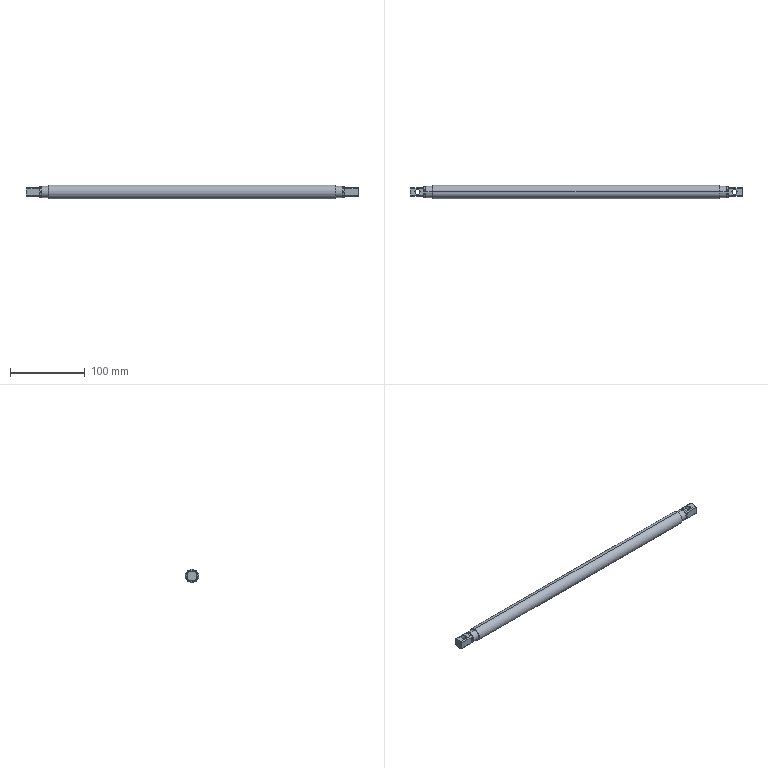Part | STEP file | PN_0017 | 1 solid | 54 faces | box 444 x 18 x 18 mm | volume 106069 mm3 | plane 24 | cylinder 18 | cone 12 | commonest cylinder face diameters 15 x8 6.8 x4 14.3 x4 18 x2